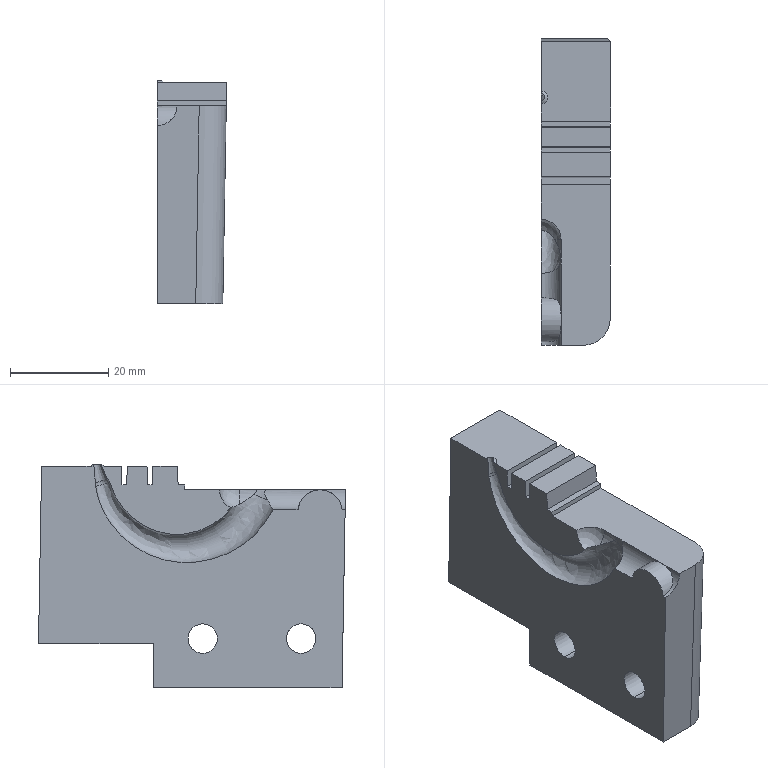Part | Creo | 1 solid | 170 faces | box 14.088 x 62.341 x 45.424 mm | volume 30992 mm3 | other 105 | plane 49 | cylinder 10 | sphere 3 | spline 2 | cone 1 | commonest cylinder face diameters 6 x4 8 x3 9 x1 11 x1 45.582 x1